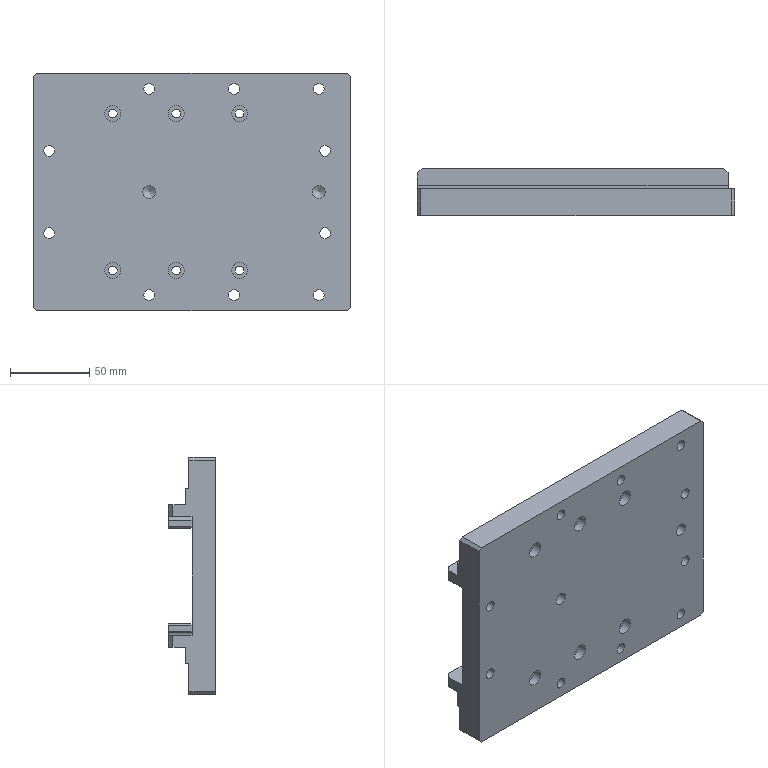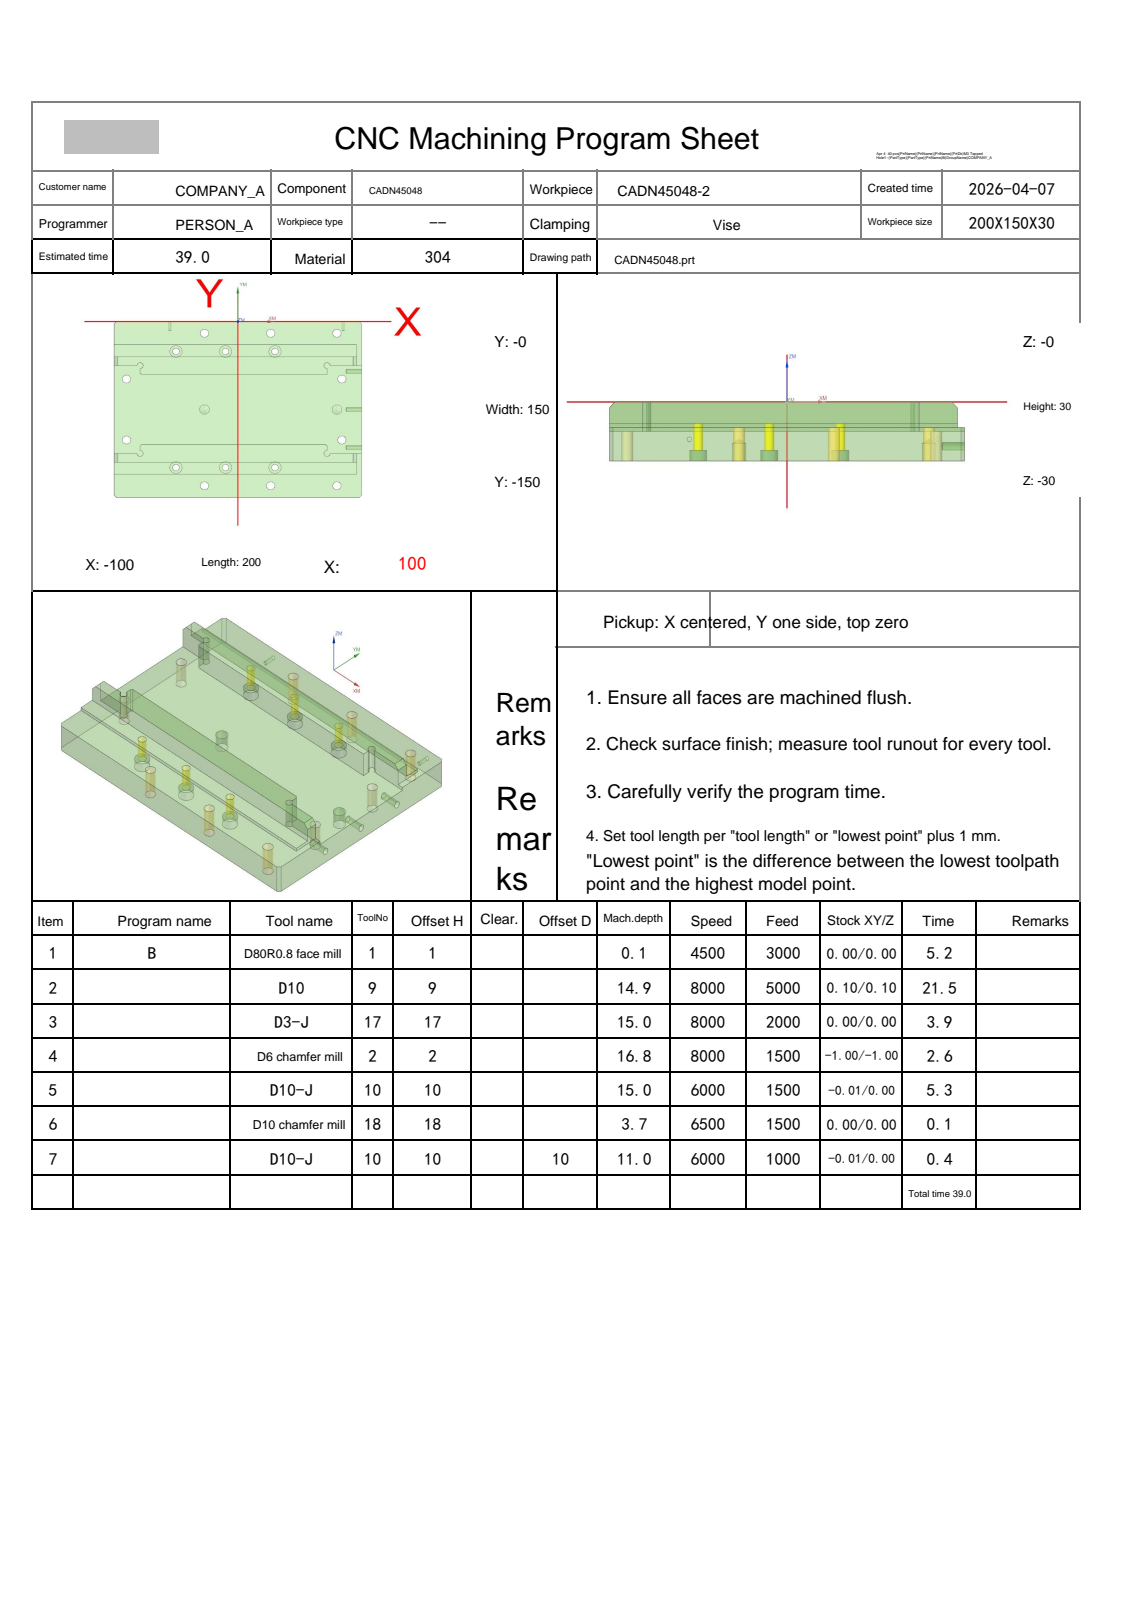NC program | NX | posted by the shop | part box 200 x 30 x 150 mm
Lines 220 to 1269 of 19220:
N2 T09 M06
(D10  D=10. R=0. H=09 ce=0.10 di=0.10)
G00 G90 G54 X114.5 Y-68. M03 S8000
G43 H09 Z14.5
M08
Z.626
G01 Z-.574 F5000.
X106.92
G03 X99.92 Y-75. I0.0 J-7.
G01 Y-107.398
Y-107.934
Y-109.294
X99.934 Y-109.34
G02 X101.02 Y-112.388 I-4.808 J-3.43
G01 X101.022 Y-130.184
X100.946 Y-131.064
X100.709 Y-131.942
X100.583 Y-132.249
X100.285 Y-132.816
X99.931 Y-133.325
X99.92 Y-133.365
Y-147.967
X97.951 Y-149.92
X-97.967
X-99.92 Y-147.957
Y-135.302
Y-134.638
Y-130.701
G02 X-99.257 Y-129.76 I1. J0.0
G01 X-93.432 Y-127.679
G03 X-92.845 Y-127.12 I-.337 J.941
G02 X-91.923 Y-126.5 I.925 J-.38
G01 X93.025
G02 X94.022 Y-127.496 I-.003 J-1.
G01 Y-129.295
G02 X93.887 Y-129.793 I-1. J.003
G03 X92.92 Y-133.365 I6.113 J-3.572
G01 Y-141.923
G02 X91.923 Y-142.92 I-1. J.003
G01 X-91.923
G02 X-92.92 Y-141.923 I.003 J1.
G01 Y-135.303
Y-134.639
Y-130.995
G02 X-92.22 Y-130.295 I.7 J0.0
X-91.981 Y-130.337 I0.0 J-.7
G01 X-83.436 Y-133.44
G03 X-83.097 Y-133.5 I.34 J.94
G01 X84.924
G02 X85.92 Y-134.496 I-.004 J-1.
G01 Y-134.924
G02 X84.924 Y-135.92 I-1. J.004
G01 X-84.924
G02 X-85.894 Y-135.148 I.004 J1.
G03 X-86.139 Y-134.692 I-.973 J-.229
G01 X-92.75 Y-127.676
G03 X-93.154 Y-127.417 I-.727 J-.686
G01 X-99.673 Y-125.185
G02 X-99.952 Y-125.037 I.324 J.946
G01 X-99.997 Y-125.021
G02 X-102.391 Y-124.373 I.225 J5.579
X-103. Y-123.997 I2.619 J4.931
G01 Y-123.599
G02 X-104.115 Y-120. I5.445 J3.659
G01 Y-112.489
G02 X-103. Y-108.888 I6.541 J-.053
G01 Y-108.552
G02 X-99.998 Y-107.48 I3.136 J-4.043
G01 X-99.914 Y-107.484
X-99.92 Y-107.4
Y-42.956
Y-42.598
X-99.914 Y-42.514
X-99.999 Y-42.518
G02 X-102.416 Y-41.857 I.087 J5.067
X-103. Y-41.469 I2.505 J4.405
G01 Y-41.112
G02 X-104.115 Y-37.5 I5.426 J3.653
G01 Y-29.984
G02 X-103. Y-26.401 I6.56 J-.077
G01 Y-26.046
G02 X-99.997 Y-24.979 I3.218 J-4.3
G01 X-99.913 Y-24.983
X-99.92 Y-24.899
Y-15.362
Y-14.698
Y-2.033
X-97.951 Y-.08
X97.967
X99.92 Y-2.043
Y-16.564
X99.934 Y-16.609
G02 X100.953 Y-19.163 I-5.145 J-3.534
G01 X100.966 Y-19.32
G02 X100.302 Y-20.261 I-1. J0.0
G01 X94.534 Y-22.321
G03 X93.947 Y-22.88 I.337 J-.941
G02 X93.025 Y-23.5 I-.925 J.38
G01 X-91.923
G02 X-92.92 Y-22.503 I.003 J1.
G01 Y-15.361
Y-14.697
Y-8.077
G02 X-91.923 Y-7.08 I1. J-.003
G01 X91.923
G02 X92.92 Y-8.077 I-.003 J-1.
G01 Y-16.564
G03 X93.433 Y-19.21 I7.08 J0.0
G01 X93.462 Y-19.36
G02 X93.062 Y-19.76 I-.4 J0.0
G01 X92.934 Y-19.739
X83.49 Y-16.552
G03 X83.172 Y-16.5 I-.319 J-.948
G01 X-84.924
G02 X-85.92 Y-15.504 I.004 J1.
G01 Y-15.36
Y-15.076
G02 X-84.924 Y-14.08 I1. J-.004
G01 X84.924
G02 X85.888 Y-14.829 I-.004 J-1.
G03 X86.179 Y-15.314 I.968 J.252
G01 X93.873 Y-22.367
G03 X94.212 Y-22.571 I.676 J.737
G01 X100.358 Y-24.767
G02 X101.021 Y-25.709 I-.337 J-.942
G01 X101.02 Y-37.614
G02 X99.937 Y-40.618 I-5.05 J.124
G01 X99.92 Y-40.668
Y-42.066
Y-42.602
Y-71.986
G02 X99.502 Y-72.799 I-1. J0.0
G01 X93.338 Y-77.201
G03 X92.92 Y-78.014 I.582 J-.813
G01 Y-105.003
G02 X91.924 Y-106. I-1. J.003
G01 X79.437
G02 X78.451 Y-105.145 I.003 J1.
G03 X78.241 Y-104.182 I-6.595 J-.94
X76.603 Y-101.411 I-6.241 J-1.818
G01 X75.294 Y-100.101
X75.185 Y-100.003
G03 X74.039 Y-99.254 I-4.252 J-5.253
X71.081 Y-98.5 I-3.04 J-5.745
G01 X-78.152
G03 X-82.603 Y-100.411 I.076 J-6.316
G01 X-83.69 Y-101.498
G03 X-85.258 Y-104.241 I4.69 J-4.5
X-85.451 Y-105.145 I6.418 J-1.848
G02 X-86.437 Y-106. I-.989 J.145
G01 X-91.431
G03 X-92.135 Y-106.445 I0.0 J-.779
G01 X-92.303 Y-106.8
X-92.343 Y-106.98
G03 X-91.923 Y-107.4 I.42 J0.0
G01 X-84.1
Y-105.649
G02 X-83.911 Y-104.625 I5.261 J-.441
X-82.673 Y-102.46 I4.912 J-1.374
G01 X-81.606 Y-101.394
G02 X-78.152 Y-99.9 I3.53 J-3.423
G01 X71.136 Y-99.902
G02 X73.39 Y-100.495 I-.136 J-5.098
X74.304 Y-101.091 I-2.457 J-4.762
G01 X74.606 Y-101.394
X75.614 Y-102.402
G02 X76.898 Y-104.578 I-3.614 J-3.598
X77.1 Y-105.648 I-5.042 J-1.507
G01 Y-107.4
X93.574
G02 X98.715 Y-112.5 I-.012 J-5.154
G01 Y-120.
G02 X93.574 Y-125.1 I-5.16 J.06
G01 X-97.574
G02 X-102.715 Y-120. I.019 J5.16
G01 Y-112.5
G02 X-97.574 Y-107.4 I5.141 J-.041
G01 X-97.521
X-91.923
G03 X-91.503 Y-106.98 I0.0 J.42
G01 X-91.544 Y-106.8
X-91.827 Y-106.202
G03 X-92.112 Y-105.981 I-.361 J-.172
G02 X-92.92 Y-105.003 I.192 J.981
G01 Y-101.503
G02 X-92.556 Y-100.732 I1. J0.0
G01 X-90.989 Y-99.438
G03 X-90.688 Y-99.015 I-.637 J.771
G01 X-89.025 Y-94.531
G02 X-86.681 Y-92.901 I2.344 J-.87
X-84.181 Y-95.401 I0.0 J-2.5
X-84.337 Y-96.27 I-2.5 J0.0
G01 X-86.411 Y-101.86
G02 X-88.755 Y-103.491 I-2.344 J.87
X-91.235 Y-101.308 I0.0 J2.5
G03 X-91.492 Y-100.756 I-.992 J-.127
G01 X-92.655 Y-99.498
G02 X-92.92 Y-98.819 I.735 J.679
G01 Y-51.181
G02 X-92.655 Y-50.502 I1. J0.0
G01 X-91.492 Y-49.243
G03 X-91.235 Y-48.692 I-.735 J.678
G02 X-88.755 Y-46.509 I2.48 J-.317
X-86.411 Y-48.14 I0.0 J-2.5
G01 X-84.337 Y-53.73
G02 X-84.181 Y-54.599 I-2.344 J-.87
X-86.681 Y-57.099 I-2.5 J0.0
X-89.025 Y-55.469 I0.0 J2.5
G01 X-90.688 Y-50.985
G03 X-90.989 Y-50.561 I-.938 J-.348
G01 X-92.557 Y-49.268
G02 X-92.92 Y-48.497 I.637 J.771
G01 Y-44.997
G02 X-91.923 Y-44. I1. J-.003
G01 X-86.437
G02 X-85.451 Y-44.855 I-.003 J-1.
G03 X-85.258 Y-45.758 I6.612 J.945
X-83.663 Y-48.529 I6.258 J1.756
G01 X-82.603 Y-49.589
G03 X-78.152 Y-51.5 I4.527 J4.405
G01 X72.
G03 X77.777 Y-47.98 I0.0 J6.5
X78.5 Y-45.292 I-5.794 J3.001
G01 Y-44.997
G02 X79.497 Y-44. I1. J-.003
G01 X91.431
G03 X92.135 Y-43.555 I0.0 J.779
G01 X92.303 Y-43.2
X92.344 Y-43.02
G03 X91.924 Y-42.6 I-.42 J0.0
G01 X77.1
Y-45.292
G02 X76.533 Y-47.337 I-5.115 J.318
X72. Y-50.1 I-4.533 J2.337
G01 X-78.152
G02 X-81.606 Y-48.606 I.076 J4.916
G01 X-82.743 Y-47.465
G02 X-83.911 Y-45.375 I3.743 J3.465
X-84.1 Y-44.351 I5.072 J1.465
G01 Y-42.6
X-97.574
G02 X-102.715 Y-37.5 I0.0 J5.141
G01 Y-30.
G02 X-97.574 Y-24.9 I5.16 J-.06
G01 X93.574
G02 X98.715 Y-30. I-.019 J-5.16
G01 Y-37.5
G02 X93.574 Y-42.6 I-5.154 J.054
G01 X91.924
G03 X91.504 Y-43.02 I0.0 J-.42
G01 X91.544 Y-43.2
X91.828 Y-43.798
G03 X92.112 Y-44.019 I.361 J.172
G02 X92.92 Y-44.997 I-.192 J-.981
G01 Y-71.986
G02 X92.502 Y-72.799 I-1. J0.0
G01 X86.339 Y-77.201
G03 X85.92 Y-78.014 I.582 J-.814
G01 Y-98.004
G02 X84.924 Y-99. I-1. J.004
G01 X84.089
G02 X83.261 Y-98.555 I.004 J1.
G03 X81.557 Y-96.465 I-11.261 J-7.445
G01 X80.244 Y-95.152
G03 X79.589 Y-94.562 I-5.94 J-5.94
X77.284 Y-93.052 I-8.656 J-10.694
X71.124 Y-91.5 I-6.285 J-11.948
G01 X-78.194
G03 X-84.445 Y-93.121 I.118 J-13.316
G02 X-84.92 Y-93.241 I-.475 J.88
X-85.92 Y-92.245 I0.0 J1.
G01 Y-57.755
G02 X-84.92 Y-56.759 I1. J-.004
X-84.445 Y-56.879 I0.0 J-1.
G03 X-78.194 Y-58.5 I6.369 J11.695
G01 X72.
G03 X83.825 Y-51.514 I0.0 J13.5
G02 X84.694 Y-51. I.874 J-.486
G01 X84.924
G02 X85.92 Y-51.996 I-.004 J-1.
G01 Y-71.986
G02 X85.502 Y-72.799 I-1. J0.0
G01 X79.339 Y-77.201
G03 X78.92 Y-78.014 I.581 J-.814
G01 Y-84.648
G02 X77.92 Y-85.644 I-1. J.004
X77.602 Y-85.592 I0.0 J1.
G03 X71.157 Y-84.5 I-6.603 J-19.407
G01 X-77.924
G02 X-78.92 Y-83.504 I.004 J1.
G01 Y-66.496
G02 X-77.924 Y-65.5 I1. J-.004
G01 X72.
G03 X77.649 Y-64.706 I0.0 J20.5
G02 X77.92 Y-64.669 I.271 J-.963
X78.92 Y-65.665 I0.0 J-1.
G01 Y-71.957
G02 X78.465 Y-72.796 I-1. J0.0
G01 X71.464 Y-77.339
G02 X70.921 Y-77.5 I-.544 J.839
G01 X-70.925
G02 X-71.92 Y-76.505 I.005 J1.
G01 Y-73.495
G02 X-70.925 Y-72.5 I1. J-.005
G01 X70.925
G02 X71.92 Y-73.495 I-.005 J-1.
G01 Y-75.
Y-75.5
G03 X78.92 Y-82.5 I7. J0.0
G01 Z.626
G00 Z3.
G01 X114.5 Y-68. F6000.
G00 Z.053
G01 Z-1.147 F5000.
X106.92
G03 X99.92 Y-75. I0.0 J-7.
G01 Y-107.398
Y-107.934
Y-109.294
X99.934 Y-109.34
G02 X101.02 Y-112.388 I-4.808 J-3.43
G01 X101.022 Y-130.184
X100.946 Y-131.064
X100.709 Y-131.942
X100.583 Y-132.249
X100.285 Y-132.816
X99.931 Y-133.325
X99.92 Y-133.365
Y-147.967
X97.951 Y-149.92
X-97.967
X-99.92 Y-147.957
Y-135.302
Y-134.638
Y-130.701
G02 X-99.257 Y-129.759 I1. J0.0
G01 X-93.432 Y-127.679
G03 X-92.845 Y-127.12 I-.337 J.941
G02 X-91.924 Y-126.5 I.925 J-.38
G01 X93.025
G02 X94.022 Y-127.496 I-.004 J-1.
G01 Y-129.295
G02 X93.887 Y-129.793 I-1. J.004
G03 X92.92 Y-133.365 I6.113 J-3.572
G01 Y-141.924
G02 X91.924 Y-142.92 I-1. J.004
G01 X-91.924
G02 X-92.92 Y-141.924 I.004 J1.
G01 Y-135.304
Y-134.639
Y-130.995
G02 X-92.22 Y-130.295 I.7 J0.0
X-91.981 Y-130.337 I0.0 J-.7
G01 X-83.436 Y-133.44
G03 X-83.097 Y-133.5 I.34 J.94
G01 X84.924
G02 X85.92 Y-134.496 I-.004 J-1.
G01 Y-134.924
G02 X84.924 Y-135.92 I-1. J.004
G01 X-84.924
G02 X-85.894 Y-135.148 I.004 J1.
G03 X-86.139 Y-134.692 I-.973 J-.229
G01 X-92.75 Y-127.676
G03 X-93.154 Y-127.416 I-.728 J-.686
G01 X-99.673 Y-125.185
G02 X-99.952 Y-125.037 I.324 J.946
G01 X-99.997 Y-125.021
G02 X-103.14 Y-123.895 I.225 J5.579
X-103.903 Y-123.057 I3.711 J4.149
X-104.689 Y-120. I5.769 J3.111
G01 Y-112.495
G02 X-103.987 Y-109.565 I6.469 J0.0
X-99.998 Y-107.48 I4.123 J-3.03
G01 X-99.914 Y-107.484
X-99.92 Y-107.4
Y-42.956
Y-42.777
Y-42.598
X-99.914 Y-42.514
X-99.999 Y-42.518
G02 X-103.919 Y-40.553 I.087 J5.067
X-104.689 Y-37.5 I5.751 J3.074
G01 Y-29.985
G02 X-103.84 Y-26.828 I6.554 J-.069
X-99.997 Y-24.979 I4.058 J-3.519
G01 X-99.913 Y-24.983
X-99.92 Y-24.899
Y-23.748
Y-15.362
Y-14.698
Y-2.033
X-97.951 Y-.08
X97.967
X99.92 Y-2.043
Y-16.564
X99.934 Y-16.609
G02 X100.953 Y-19.163 I-5.145 J-3.534
G01 X100.966 Y-19.32
G02 X100.302 Y-20.262 I-1. J0.0
G01 X94.533 Y-22.321
G03 X93.946 Y-22.881 I.337 J-.941
G02 X93.025 Y-23.5 I-.925 J.381
G01 X-91.924
G02 X-92.92 Y-22.504 I.004 J1.
G01 Y-15.361
Y-14.696
Y-8.076
G02 X-91.924 Y-7.08 I1. J-.004
G01 X91.924
G02 X92.92 Y-8.076 I-.004 J-1.
G01 Y-16.564
G03 X93.433 Y-19.21 I7.08 J0.0
G01 X93.462 Y-19.36
G02 X93.062 Y-19.76 I-.4 J0.0
G01 X92.934 Y-19.739
X83.49 Y-16.552
G03 X83.172 Y-16.5 I-.319 J-.948
G01 X-84.924
G02 X-85.92 Y-15.504 I.004 J1.
G01 Y-15.36
Y-15.076
G02 X-84.924 Y-14.08 I1. J-.004
G01 X84.924
G02 X85.888 Y-14.829 I-.004 J-1.
G03 X86.179 Y-15.314 I.968 J.252
G01 X93.873 Y-22.367
G03 X94.212 Y-22.572 I.676 J.737
G01 X100.358 Y-24.768
G02 X101.021 Y-25.709 I-.337 J-.942
G01 X101.02 Y-37.614
G02 X99.937 Y-40.618 I-5.05 J.124
G01 X99.92 Y-40.668
Y-42.066
Y-42.602
Y-71.986
G02 X99.502 Y-72.799 I-1. J0.0
G01 X93.338 Y-77.201
G03 X92.92 Y-78.014 I.582 J-.813
G01 Y-105.004
G02 X91.924 Y-106. I-1. J.004
G01 X79.437
G02 X78.452 Y-105.145 I.004 J1.
G03 X78.241 Y-104.182 I-6.596 J-.94
X76.603 Y-101.411 I-6.241 J-1.818
G01 X75.294 Y-100.101
X75.185 Y-100.003
G03 X74.039 Y-99.254 I-4.252 J-5.253
X71.081 Y-98.5 I-3.04 J-5.745
G01 X-78.174
G03 X-82.603 Y-100.411 I.098 J-6.316
G01 X-83.774 Y-101.589
G03 X-85.258 Y-104.241 I4.774 J-4.411
X-85.451 Y-105.145 I6.418 J-1.848
G02 X-86.437 Y-106. I-.989 J.145
G01 X-91.431
G03 X-92.135 Y-106.445 I0.0 J-.779
G01 X-92.303 Y-106.8
X-92.344 Y-106.98
G03 X-91.924 Y-107.4 I.42 J0.0
G01 X-84.1
Y-105.999
Y-105.649
G02 X-83.911 Y-104.625 I5.261 J-.441
X-82.606 Y-102.394 I4.912 J-1.376
G01 X-81.606 Y-101.394
G02 X-78.152 Y-99.9 I3.53 J-3.423
G01 X-78.
X71.136 Y-99.902
G02 X73.39 Y-100.495 I-.136 J-5.098
X74.304 Y-101.091 I-2.457 J-4.762
G01 X74.606 Y-101.394
X75.614 Y-102.402
G02 X76.898 Y-104.578 I-3.614 J-3.598
X77.1 Y-105.648 I-5.042 J-1.507
G01 Y-106.
Y-107.4
X94.147
X94.168
G02 X99.289 Y-112.5 I0.0 J-5.121
G01 Y-120.
G02 X94.168 Y-125.1 I-5.121 J.021
G01 X94.147
X-98.147
G02 X-103.289 Y-120. I.012 J5.154
G01 Y-112.495
G02 X-98.658 Y-107.444 I5.069 J0.0
G01 X-98.147 Y-107.4
X-91.924
G03 X-91.504 Y-106.98 I0.0 J.42
G01 X-91.544 Y-106.8
X-91.828 Y-106.202
G03 X-92.112 Y-105.981 I-.361 J-.172
G02 X-92.92 Y-105.004 I.192 J.981
G01 Y-101.498
G02 X-92.556 Y-100.727 I1. J0.0
G01 X-90.99 Y-99.435
G03 X-90.69 Y-99.014 I-.636 J.771
G01 X-89.018 Y-94.529
G02 X-86.675 Y-92.903 I2.342 J-.873
X-84.175 Y-95.403 I0.0 J-2.5
X-84.333 Y-96.276 I-2.5 J0.0
G01 X-86.416 Y-101.864
G02 X-88.759 Y-103.49 I-2.342 J.873
X-91.239 Y-101.303 I0.0 J2.5
G03 X-91.496 Y-100.75 I-.992 J-.125
G01 X-92.655 Y-99.495
G02 X-92.92 Y-98.817 I.735 J.678
G01 Y-51.181
G02 X-92.655 Y-50.502 I1. J0.0
G01 X-91.492 Y-49.243
G03 X-91.235 Y-48.692 I-.735 J.678
G02 X-88.755 Y-46.509 I2.48 J-.317
X-86.411 Y-48.14 I0.0 J-2.5
G01 X-84.337 Y-53.73
G02 X-84.181 Y-54.599 I-2.344 J-.87
X-86.681 Y-57.099 I-2.5 J0.0
X-89.025 Y-55.469 I0.0 J2.5
G01 X-90.688 Y-50.985
G03 X-90.989 Y-50.561 I-.938 J-.348
G01 X-92.557 Y-49.268
G02 X-92.92 Y-48.497 I.637 J.771
G01 Y-44.996
G02 X-91.924 Y-44. I1. J-.004
G01 X-86.437
G02 X-85.451 Y-44.855 I-.004 J-1.
G03 X-85.258 Y-45.758 I6.612 J.945
X-83.663 Y-48.529 I6.258 J1.756
G01 X-82.603 Y-49.589
G03 X-78.152 Y-51.5 I4.527 J4.405
G01 X72.
G03 X77.777 Y-47.98 I0.0 J6.5
X78.5 Y-45.292 I-5.794 J3.001
G01 Y-44.996
G02 X79.496 Y-44. I1. J-.004
G01 X91.431
G03 X92.135 Y-43.555 I0.0 J.779
G01 X92.303 Y-43.2
X92.344 Y-43.02
G03 X91.924 Y-42.6 I-.42 J0.0
G01 X77.1
Y-45.292
G02 X76.533 Y-47.337 I-5.115 J.318
X72. Y-50.1 I-4.533 J2.337
G01 X-78.152
G02 X-81.606 Y-48.606 I.076 J4.916
G01 X-82.743 Y-47.465
G02 X-83.911 Y-45.375 I3.743 J3.465
X-84.1 Y-44.351 I5.072 J1.465
G01 Y-44.
Y-42.6
X-98.147
X-98.168
G02 X-103.289 Y-37.5 I0.0 J5.121
G01 Y-30.
G02 X-98.147 Y-24.9 I5.154 J-.054
G01 X94.147
X94.168
G02 X99.289 Y-30. I0.0 J-5.121
G01 Y-37.5
G02 X94.168 Y-42.6 I-5.121 J.021
G01 X94.147
X91.924
G03 X91.504 Y-43.02 I0.0 J-.42
G01 X91.544 Y-43.2
X91.828 Y-43.798
G03 X92.112 Y-44.019 I.361 J.172
G02 X92.92 Y-44.996 I-.192 J-.981
G01 Y-71.986
G02 X92.502 Y-72.799 I-1. J0.0
G01 X86.339 Y-77.201
G03 X85.92 Y-78.014 I.582 J-.814
G01 Y-98.004
G02 X84.924 Y-99. I-1. J.004
G01 X84.089
G02 X83.262 Y-98.555 I.004 J1.
G03 X81.557 Y-96.465 I-11.262 J-7.445
G01 X80.244 Y-95.152
G03 X79.589 Y-94.562 I-5.94 J-5.94
X77.284 Y-93.052 I-8.656 J-10.694
X71.124 Y-91.5 I-6.285 J-11.948
G01 X-78.228
G03 X-84.446 Y-93.121 I.152 J-13.316
G02 X-84.92 Y-93.241 I-.474 J.88
X-85.92 Y-92.245 I0.0 J1.
G01 Y-57.755
G02 X-84.92 Y-56.759 I1. J-.004
X-84.446 Y-56.878 I0.0 J-1.
G03 X-78.194 Y-58.5 I6.369 J11.695
G01 X72.
G03 X83.825 Y-51.514 I0.0 J13.5
G02 X84.694 Y-51. I.874 J-.486
G01 X84.924
G02 X85.92 Y-51.996 I-.004 J-1.
G01 Y-71.986
G02 X85.502 Y-72.799 I-1. J0.0
G01 X79.339 Y-77.201
G03 X78.92 Y-78.014 I.582 J-.814
G01 Y-84.648
G02 X77.92 Y-85.644 I-1. J.005
X77.602 Y-85.592 I0.0 J1.
G03 X71.157 Y-84.5 I-6.604 J-19.407
G01 X-77.925
G02 X-78.92 Y-83.505 I.005 J1.
G01 Y-66.495
G02 X-77.925 Y-65.5 I1. J-.005
G01 X72.
G03 X77.649 Y-64.706 I0.0 J20.5
G02 X77.92 Y-64.669 I.271 J-.963
X78.92 Y-65.664 I0.0 J-1.
G01 Y-71.957
G02 X78.465 Y-72.796 I-1. J0.0
G01 X71.464 Y-77.339
G02 X70.921 Y-77.5 I-.544 J.839
G01 X-70.925
G02 X-71.92 Y-76.505 I.005 J1.
G01 Y-73.495
G02 X-70.925 Y-72.5 I1. J-.005
G01 X70.925
G02 X71.92 Y-73.495 I-.005 J-1.
G01 Y-75.
Y-75.5
G03 X78.92 Y-82.5 I7. J0.0
G01 Z.053
G00 Z3.
G01 X114.5 Y-68. F6000.
G00 Z-.521
G01 Z-1.721 F5000.
X106.92
G03 X99.92 Y-75. I0.0 J-7.
G01 Y-107.398
Y-107.934
Y-109.294
X99.934 Y-109.34
G02 X101.02 Y-112.388 I-4.808 J-3.43
G01 X101.022 Y-130.184
X100.946 Y-131.064
X100.709 Y-131.942
X100.583 Y-132.249
X100.285 Y-132.816
X99.931 Y-133.325
X99.92 Y-133.365
Y-147.967
X97.951 Y-149.92
X-97.967
X-99.92 Y-147.957
Y-135.302
Y-134.638
Y-130.7
G02 X-99.257 Y-129.759 I1. J0.0
G01 X-93.431 Y-127.678
G03 X-92.845 Y-127.119 I-.337 J.941
G02 X-91.924 Y-126.5 I.925 J-.381
G01 X93.026
G02 X94.022 Y-127.496 I-.004 J-1.
G01 Y-129.296
G02 X93.888 Y-129.792 I-1. J.004
G03 X92.92 Y-133.365 I6.112 J-3.573
G01 Y-141.924
G02 X91.924 Y-142.92 I-1. J.004
G01 X-91.924
G02 X-92.92 Y-141.924 I.004 J1.
G01 Y-135.303
Y-134.639
Y-130.995
G02 X-92.22 Y-130.295 I.7 J0.0
X-91.981 Y-130.337 I0.0 J-.7
G01 X-83.436 Y-133.44
G03 X-83.097 Y-133.5 I.34 J.94
G01 X84.925
G02 X85.92 Y-134.495 I-.005 J-1.
G01 Y-134.925
G02 X84.925 Y-135.92 I-1. J.005
G01 X-84.925
G02 X-85.894 Y-135.148 I.005 J1.
G03 X-86.138 Y-134.693 I-.973 J-.229
G01 X-92.75 Y-127.676
G03 X-93.154 Y-127.416 I-.728 J-.686
G01 X-99.673 Y-125.185
G02 X-99.952 Y-125.037 I.324 J.946
G01 X-99.997 Y-125.021
G02 X-103. Y-123.997 I.225 J5.579
G01 X-103.14 Y-123.895
G02 X-104.996 Y-119.745 I3.711 J4.15
X-104.991 Y-119.506 I5.567 J0.0
G01 X-104.977 Y-112.387
G02 X-99.998 Y-107.48 I5.112 J-.208
G01 X-99.914 Y-107.484
X-99.92 Y-107.4
Y-43.893
Y-42.956
Y-42.598
X-99.914 Y-42.514
X-99.999 Y-42.518
G02 X-103. Y-41.469 I.087 J5.067
X-104.977 Y-37.614 I3.089 J4.018
G01 X-104.991 Y-30.495
X-104.958 Y-29.612
X-104.807 Y-28.734
X-104.494 Y-27.856
X-104.151 Y-27.222
G02 X-103. Y-26.046 I4.369 J-3.124
X-99.997 Y-24.979 I3.218 J-4.3
G01 X-99.913 Y-24.983
X-99.92 Y-24.899
Y-15.362
Y-14.698
Y-2.033
X-97.951 Y-.08
X97.967
X99.92 Y-2.043
Y-16.564
X99.934 Y-16.609
G02 X100.953 Y-19.164 I-5.145 J-3.534
G01 X100.966 Y-19.32
G02 X100.302 Y-20.262 I-1. J0.0
G01 X94.533 Y-22.322
G03 X93.946 Y-22.881 I.337 J-.941
G02 X93.026 Y-23.5 I-.925 J.381
G01 X-91.924
G02 X-92.92 Y-22.504 I.004 J1.
G01 Y-15.361
Y-14.697
Y-8.076
G02 X-91.924 Y-7.08 I1. J-.004
G01 X91.924
G02 X92.92 Y-8.076 I-.004 J-1.
G01 Y-16.564
G03 X93.433 Y-19.211 I7.08 J0.0
G01 X93.462 Y-19.36
G02 X93.062 Y-19.76 I-.4 J0.0
G01 X92.935 Y-19.739
X83.49 Y-16.552
G03 X83.172 Y-16.5 I-.319 J-.948
G01 X-84.925
G02 X-85.92 Y-15.505 I.005 J1.
G01 Y-15.36
Y-15.076
G02 X-84.925 Y-14.08 I1. J-.004
G01 X84.925
G02 X85.888 Y-14.829 I-.005 J-1.
G03 X86.179 Y-15.313 I.968 J.252
G01 X93.873 Y-22.368
G03 X94.212 Y-22.572 I.676 J.737
G01 X100.358 Y-24.768
G02 X101.021 Y-25.709 I-.337 J-.942
G01 Y-28.293
X101.02 Y-37.614
G02 X99.937 Y-40.618 I-5.05 J.124
G01 X99.92 Y-40.668
Y-42.066
Y-42.602
Y-71.986
G02 X99.502 Y-72.799 I-1. J0.0
G01 X93.338 Y-77.201
G03 X92.92 Y-78.014 I.582 J-.813
G01 Y-105.004
G02 X91.924 Y-106. I-1. J.004
G01 X79.437
G02 X78.452 Y-105.146 I.004 J1.
G03 X78.241 Y-104.182 I-6.596 J-.939
X76.603 Y-101.411 I-6.241 J-1.818
G01 X75.294 Y-100.101
X75.185 Y-100.003
G03 X74.039 Y-99.254 I-4.252 J-5.253
X72.554 Y-98.689 I-3.039 J-5.746
X71.081 Y-98.5 I-1.556 J-6.311
G01 X-78.174
G03 X-82.603 Y-100.411 I.098 J-6.316
G01 X-83.774 Y-101.589
G03 X-85.258 Y-104.241 I4.774 J-4.411
X-85.451 Y-105.146 I6.418 J-1.848
G02 X-86.436 Y-106. I-.989 J.146
G01 X-91.432
G03 X-92.135 Y-106.445 I0.0 J-.779
G01 X-92.304 Y-106.8
X-92.344 Y-106.98
G03 X-91.924 Y-107.4 I.42 J0.0
G01 X-84.1
Y-105.999
Y-105.649
G02 X-83.911 Y-104.625 I5.261 J-.441
X-82.606 Y-102.394 I4.912 J-1.376
G01 X-81.606 Y-101.394
G02 X-78.152 Y-99.9 I3.53 J-3.423
G01 X-78.
X71.136 Y-99.902
G02 X73.39 Y-100.495 I-.136 J-5.098
X74.304 Y-101.091 I-2.457 J-4.762
G01 X74.606 Y-101.394
X75.614 Y-102.402
G02 X76.898 Y-104.578 I-3.614 J-3.598
X77.1 Y-105.648 I-5.042 J-1.507
G01 Y-106.
Y-107.4
X94.721
X94.742
G02 X99.862 Y-112.5 I0.0 J-5.121
G01 Y-120.
G02 X94.721 Y-125.1 I-5.156 J.056
G01 X-98.721
G02 X-103.862 Y-120. I.012 J5.154
G01 Y-112.5
G02 X-98.742 Y-107.4 I5.121 J-.021
G01 X-98.721
X-91.924
G03 X-91.504 Y-106.98 I0.0 J.42
G01 X-91.545 Y-106.8
X-91.828 Y-106.202
G03 X-92.112 Y-105.981 I-.361 J-.172
G02 X-92.92 Y-105.004 I.192 J.981
G01 Y-101.498
G02 X-92.556 Y-100.727 I1. J0.0
G01 X-90.99 Y-99.435
G03 X-90.69 Y-99.014 I-.636 J.771
G01 X-89.018 Y-94.529
G02 X-86.675 Y-92.903 I2.342 J-.873
X-84.175 Y-95.403 I0.0 J-2.5
X-84.333 Y-96.276 I-2.5 J0.0
G01 X-86.416 Y-101.864
G02 X-88.759 Y-103.49 I-2.342 J.873
X-91.239 Y-101.303 I0.0 J2.5
G03 X-91.496 Y-100.75 I-.992 J-.125
G01 X-92.655 Y-99.495
G02 X-92.92 Y-98.817 I.735 J.678
G01 Y-51.181
G02 X-92.655 Y-50.502 I1. J0.0
G01 X-91.492 Y-49.243
G03 X-91.235 Y-48.692 I-.735 J.678
G02 X-88.755 Y-46.509 I2.48 J-.317
X-86.411 Y-48.14 I0.0 J-2.5
G01 X-84.337 Y-53.73
G02 X-84.181 Y-54.599 I-2.344 J-.87
X-86.681 Y-57.099 I-2.5 J0.0
X-89.025 Y-55.469 I0.0 J2.5
G01 X-90.688 Y-50.985
G03 X-90.989 Y-50.561 I-.938 J-.348
G01 X-92.557 Y-49.268
G02 X-92.92 Y-48.497 I.637 J.771
G01 Y-44.996
G02 X-91.924 Y-44. I1. J-.004
G01 X-86.436
G02 X-85.451 Y-44.854 I-.004 J-1.
G03 X-85.258 Y-45.758 I6.612 J.944
X-83.663 Y-48.529 I6.258 J1.756
G01 X-82.603 Y-49.589
G03 X-78.152 Y-51.5 I4.527 J4.405
G01 X72.
G03 X77.777 Y-47.98 I0.0 J6.5
X78.5 Y-45.292 I-5.794 J3.001
G01 Y-44.996
G02 X79.496 Y-44. I1. J-.004
G01 X91.432
G03 X92.135 Y-43.555 I0.0 J.779
G01 X92.304 Y-43.2
X92.344 Y-43.02
G03 X91.924 Y-42.6 I-.42 J0.0
G01 X77.1
Y-45.001
Y-45.292
G02 X76.533 Y-47.337 I-5.115 J.318
X72. Y-50.1 I-4.533 J2.337
G01 X-78.152
G02 X-81.606 Y-48.606 I.076 J4.916
G01 X-82.743 Y-47.465
G02 X-83.911 Y-45.375 I3.743 J3.465
X-84.1 Y-44.351 I5.072 J1.465
G01 Y-44.
Y-42.6
X-98.721
X-98.742
G02 X-103.862 Y-37.5 I0.0 J5.121
G01 Y-30.
G02 X-98.721 Y-24.9 I5.154 J-.054
G01 X94.721
G02 X99.862 Y-30. I-.015 J-5.156
G01 Y-37.5
G02 X94.742 Y-42.6 I-5.121 J.021
G01 X94.721
X91.924
G03 X91.504 Y-43.02 I0.0 J-.42
G01 X91.545 Y-43.2
X91.828 Y-43.798
G03 X92.112 Y-44.019 I.361 J.172
G02 X92.92 Y-44.996 I-.192 J-.981
G01 Y-71.986
G02 X92.502 Y-72.799 I-1. J0.0
G01 X86.339 Y-77.201
G03 X85.92 Y-78.014 I.582 J-.814
G01 Y-98.005
G02 X84.925 Y-99. I-1. J.005
G01 X84.089
G02 X83.262 Y-98.555 I.005 J1.
G03 X81.557 Y-96.465 I-11.262 J-7.445
G01 X80.244 Y-95.152
G03 X79.589 Y-94.562 I-5.94 J-5.94
X77.284 Y-93.051 I-8.656 J-10.694
X74.229 Y-91.892 I-6.284 J-11.949
X71.125 Y-91.5 I-3.231 J-13.108
G01 X-78.228
G03 X-84.446 Y-93.122 I.152 J-13.316
G02 X-84.92 Y-93.241 I-.474 J.88
X-85.92 Y-92.246 I0.0 J1.
G01 Y-57.754
G02 X-84.92 Y-56.759 I1. J-.005
X-84.446 Y-56.878 I0.0 J-1.
G03 X-78.194 Y-58.5 I6.37 J11.695
G01 X72.
G03 X83.825 Y-51.513 I0.0 J13.5
G02 X84.694 Y-51. I.874 J-.487
G01 X84.925
G02 X85.92 Y-51.995 I-.005 J-1.
G01 Y-71.986
G02 X85.502 Y-72.799 I-1. J0.0
G01 X79.339 Y-77.201
G03 X78.92 Y-78.014 I.581 J-.814
G01 Y-84.649
G02 X77.92 Y-85.644 I-1. J.005
X77.603 Y-85.592 I0.0 J1.
G03 X75.904 Y-85.095 I-6.603 J-19.408
X71.192 Y-84.5 I-4.906 J-19.904
G01 X-77.925
G02 X-78.92 Y-83.505 I.005 J1.
G01 Y-66.495
G02 X-77.925 Y-65.5 I1. J-.005
G01 X72.
G03 X77.649 Y-64.706 I0.0 J20.5
G02 X77.92 Y-64.669 I.271 J-.963
X78.92 Y-65.664 I0.0 J-1.
G01 Y-71.957
G02 X78.465 Y-72.796 I-1. J0.0
G01 X71.464 Y-77.34
G02 X70.921 Y-77.5 I-.544 J.839
G01 X-70.925
G02 X-71.92 Y-76.506 I.005 J1.
G01 Y-73.495
G02 X-70.925 Y-72.5 I1. J-.005
G01 X70.925
G02 X71.92 Y-73.495 I-.005 J-1.
G01 Y-75.
Y-75.5
G03 X78.92 Y-82.5 I7. J0.0
G01 Z-.521
G00 Z3.
G01 X114.5 Y-68. F6000.
G00 Z-1.095
G01 Z-2.295 F5000.
X106.92
G03 X99.92 Y-75. I0.0 J-7.
G01 Y-107.398
Y-107.934
Y-109.294
X99.934 Y-109.34
G02 X101.02 Y-112.388 I-4.808 J-3.43
G01 X101.022 Y-130.184
X100.946 Y-131.064
X100.709 Y-131.942
X100.583 Y-132.249
X100.285 Y-132.816
X99.934 Y-133.319
X99.92 Y-133.365
Y-147.967
X97.951 Y-149.92
X-97.967
X-99.92 Y-147.957
Y-135.302
Y-134.638
Y-125.101
X-99.932 Y-125.059
G03 X-99.295 Y-125.1 I.652 J5.115
G01 X91.927
G02 X92.927 Y-126.1 I0.0 J-1.
G01 X92.914 Y-126.267
X92.066 Y-131.282
X92.052 Y-131.448
G03 X92.488 Y-132.274 I1. J0.0
G02 X92.924 Y-133.1 I-.564 J-.826
G01 Y-133.13
G03 X92.92 Y-133.365 I7.076 J-.235
G01 Y-141.923
G02 X91.923 Y-142.92 I-1. J.003
G01 X-91.923
G02 X-92.92 Y-141.923 I.003 J1.
G01 Y-135.304
Y-134.639
Y-133.097
G02 X-91.923 Y-132.1 I1. J-.003
G01 X88.465
G02 X89.265 Y-132.9 I0.0 J-.8
G01 X89.252 Y-133.046
X88.433 Y-137.452
X88.418 Y-137.573
G02 X87.524 Y-138.42 I-.898 J.053
G01 X-87.524
G02 X-88.42 Y-137.52 I.004 J.9
G01 Y-137.497
G02 X-87.524 Y-136.6 I.9 J-.003
G01 X85.316
G03 X85.896 Y-136.414 I-.001 J1.
G01 X91.419 Y-132.463
G03 X91.837 Y-131.65 I-.582 J.813
G01 X91.823 Y-131.484
X90.941 Y-126.267
X90.927 Y-126.1
G02 X91.927 Y-125.1 I1. J0.0
G01 X95.295
X95.315
G03 X100.436 Y-120. I0.0 J5.121
G01 Y-112.5
G03 X95.315 Y-107.4 I-5.121 J-.021
G01 X95.295
X77.1
Y-105.999
Y-105.648
G03 X76.898 Y-104.578 I-5.244 J-.437
X75.606 Y-102.394 I-4.898 J-1.422
G01 X74.605 Y-101.393
X74.304 Y-101.091
G03 X73.39 Y-100.495 I-3.371 J-4.165
X71. Y-99.9 I-2.39 J-4.506
G01 X-78.152
G03 X-81.636 Y-101.424 I.075 J-4.917
G01 X-82.743 Y-102.536
G03 X-83.911 Y-104.625 I3.743 J-3.464
X-84.1 Y-105.649 I5.072 J-1.465
G01 Y-106.
Y-107.4
X-99.295
X-99.315
G03 X-99.929 Y-107.437 I0.0 J-5.121
G01 X-99.92 Y-107.4
Y-42.956
Y-42.598
X-99.928 Y-42.563
G03 X-99.315 Y-42.6 I.612 J5.084
G01 X-99.295
X-84.1
Y-44.001
Y-44.351
G03 X-83.911 Y-45.375 I5.261 J.441
X-83.406 Y-46.568 I4.911 J1.375
X-82.606 Y-47.606 I4.407 J2.569
G01 X-81.587 Y-48.626
G03 X-78.152 Y-50.1 I3.511 J3.442
G01 X-78.
X72.
G03 X76.533 Y-47.337 I0.0 J5.1
X77.1 Y-45.292 I-4.549 J2.362
G01 Y-45.
Y-42.6
X95.295